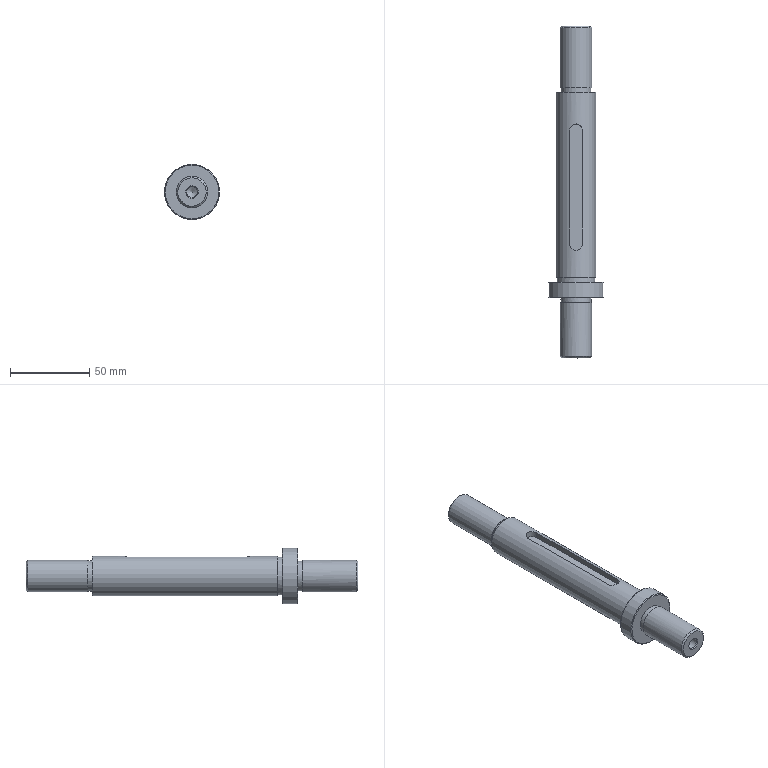Part | STEP file | 冲床-300配套压波_id574_x_t | 1 solid | 30 faces | box 35 x 210 x 35 mm | volume 89544 mm3 | plane 11 | cylinder 11 | cone 8 | commonest cylinder face diameters 6.8 x2 8.04 x2 19 x2 20 x2 24 x1 25 x1
STEP:
#1=CARTESIAN_POINT('',(1267.,-67.,172.35));
#2=VERTEX_POINT('',#1);
#3=CARTESIAN_POINT('',(1250.,-67.,172.35));
#4=DIRECTION('',(0.,-1.,0.));
#5=DIRECTION('',(1.,0.,0.));
#6=AXIS2_PLACEMENT_3D('',#3,#4,#5);
#7=CIRCLE('',#6,17.);
#8=EDGE_CURVE('',#2,#2,#7,.T.);
#9=ORIENTED_EDGE('',*,*,#8,.T.);
#10=EDGE_LOOP('',(#9));
#11=FACE_BOUND('',#10,.T.);
#12=CARTESIAN_POINT('',(1259.5,-67.,172.35));
#13=VERTEX_POINT('',#12);
#14=CARTESIAN_POINT('',(1250.,-67.,172.35));
#15=DIRECTION('',(0.,-1.,0.));
#16=DIRECTION('',(1.,0.,0.));
#17=AXIS2_PLACEMENT_3D('',#14,#15,#16);
#18=CIRCLE('',#17,9.5);
#19=EDGE_CURVE('',#13,#13,#18,.T.);
#20=ORIENTED_EDGE('',*,*,#19,.F.);
#21=EDGE_LOOP('',(#20));
#22=FACE_BOUND('',#21,.T.);
#23=CARTESIAN_POINT('',(1250.,-67.,172.35));
#24=DIRECTION('',(0.,-1.,0.));
#25=DIRECTION('',(1.,0.,0.));
#26=AXIS2_PLACEMENT_3D('',#23,#24,#25);
#27=PLANE('',#26);
#28=ADVANCED_FACE('',(#11,#22),#27,.T.);
#29=CARTESIAN_POINT('',(1233.,-57.,172.35));
#30=VERTEX_POINT('',#29);
#31=CARTESIAN_POINT('',(1250.,-57.,172.35));
#32=DIRECTION('',(0.,1.,0.));
#33=DIRECTION('',(-1.,0.,0.));
#34=AXIS2_PLACEMENT_3D('',#31,#32,#33);
#35=CIRCLE('',#34,17.);
#36=EDGE_CURVE('',#30,#30,#35,.T.);
#37=ORIENTED_EDGE('',*,*,#36,.T.);
#38=EDGE_LOOP('',(#37));
#39=FACE_BOUND('',#38,.T.);
#40=CARTESIAN_POINT('',(1238.,-57.,172.35));
#41=VERTEX_POINT('',#40);
#42=CARTESIAN_POINT('',(1250.,-57.,172.35));
#43=DIRECTION('',(0.,1.,0.));
#44=DIRECTION('',(-1.,0.,0.));
#45=AXIS2_PLACEMENT_3D('',#42,#43,#44);
#46=CIRCLE('',#45,12.);
#47=EDGE_CURVE('',#41,#41,#46,.T.);
#48=ORIENTED_EDGE('',*,*,#47,.F.);
#49=EDGE_LOOP('',(#48));
#50=FACE_BOUND('',#49,.T.);
#51=CARTESIAN_POINT('',(1250.,-57.,172.35));
#52=DIRECTION('',(0.,1.,0.));
#53=DIRECTION('',(-1.,0.,0.));
#54=AXIS2_PLACEMENT_3D('',#51,#52,#53);
#55=PLANE('',#54);
#56=ADVANCED_FACE('',(#39,#50),#55,.T.);
#57=CARTESIAN_POINT('',(1250.,-66.5,189.85));
#58=VERTEX_POINT('',#57);
#59=CARTESIAN_POINT('',(1250.,-66.5,172.35));
#60=DIRECTION('',(0.,1.,0.));
#61=DIRECTION('',(0.,0.,1.));
#62=AXIS2_PLACEMENT_3D('',#59,#60,#61);
#63=CIRCLE('',#62,17.5);
#64=EDGE_CURVE('',#58,#58,#63,.T.);
#65=ORIENTED_EDGE('',*,*,#64,.T.);
#66=EDGE_LOOP('',(#65));
#67=FACE_BOUND('',#66,.T.);
#68=CARTESIAN_POINT('',(1250.,-57.5,154.85));
#69=VERTEX_POINT('',#68);
#70=CARTESIAN_POINT('',(1250.,-57.5,172.35));
#71=DIRECTION('',(0.,-1.,0.));
#72=DIRECTION('',(0.,0.,-1.));
#73=AXIS2_PLACEMENT_3D('',#70,#71,#72);
#74=CIRCLE('',#73,17.5);
#75=EDGE_CURVE('',#69,#69,#74,.T.);
#76=ORIENTED_EDGE('',*,*,#75,.T.);
#77=EDGE_LOOP('',(#76));
#78=FACE_BOUND('',#77,.T.);
#79=CARTESIAN_POINT('',(1250.,-54.,172.35));
#80=DIRECTION('',(0.,-1.,0.));
#81=DIRECTION('',(1.,0.,0.));
#82=AXIS2_PLACEMENT_3D('',#79,#80,#81);
#83=CYLINDRICAL_SURFACE('',#82,17.5);
#84=ADVANCED_FACE('',(#67,#78),#83,.T.);
#85=ORIENTED_EDGE('',*,*,#8,.F.);
#86=EDGE_LOOP('',(#85));
#87=FACE_BOUND('',#86,.T.);
#88=ORIENTED_EDGE('',*,*,#64,.F.);
#89=EDGE_LOOP('',(#88));
#90=FACE_BOUND('',#89,.T.);
#91=CARTESIAN_POINT('',(1250.,-66.5,172.35));
#92=DIRECTION('',(0.,1.,0.));
#93=DIRECTION('',(0.,0.,1.));
#94=AXIS2_PLACEMENT_3D('',#91,#92,#93);
#95=CONICAL_SURFACE('',#94,17.5,45.);
#96=ADVANCED_FACE('',(#87,#90),#95,.T.);
#97=ORIENTED_EDGE('',*,*,#36,.F.);
#98=EDGE_LOOP('',(#97));
#99=FACE_BOUND('',#98,.T.);
#100=ORIENTED_EDGE('',*,*,#75,.F.);
#101=EDGE_LOOP('',(#100));
#102=FACE_BOUND('',#101,.T.);
#103=CARTESIAN_POINT('',(1250.,-57.5,172.35));
#104=DIRECTION('',(0.,-1.,0.));
#105=DIRECTION('',(0.,0.,-1.));
#106=AXIS2_PLACEMENT_3D('',#103,#104,#105);
#107=CONICAL_SURFACE('',#106,17.5,45.);
#108=ADVANCED_FACE('',(#99,#102),#107,.T.);
#109=CARTESIAN_POINT('',(1250.,-54.,160.35));
#110=VERTEX_POINT('',#109);
#111=CARTESIAN_POINT('',(1250.,-54.,172.35));
#112=DIRECTION('',(0.,-1.,0.));
#113=DIRECTION('',(0.,0.,-1.));
#114=AXIS2_PLACEMENT_3D('',#111,#112,#113);
#115=CIRCLE('',#114,12.);
#116=EDGE_CURVE('',#110,#110,#115,.T.);
#117=ORIENTED_EDGE('',*,*,#116,.F.);
#118=EDGE_LOOP('',(#117));
#119=FACE_BOUND('',#118,.T.);
#120=CARTESIAN_POINT('',(1250.,-54.,159.85));
#121=VERTEX_POINT('',#120);
#122=CARTESIAN_POINT('',(1250.,-54.,172.35));
#123=DIRECTION('',(0.,1.,0.));
#124=DIRECTION('',(0.,0.,-1.));
#125=AXIS2_PLACEMENT_3D('',#122,#123,#124);
#126=CIRCLE('',#125,12.5);
#127=EDGE_CURVE('',#121,#121,#126,.T.);
#128=ORIENTED_EDGE('',*,*,#127,.F.);
#129=EDGE_LOOP('',(#128));
#130=FACE_BOUND('',#129,.T.);
#131=CARTESIAN_POINT('',(1250.,-54.,172.35));
#132=DIRECTION('',(0.,-1.,0.));
#133=DIRECTION('',(0.,0.,-1.));
#134=AXIS2_PLACEMENT_3D('',#131,#132,#133);
#135=PLANE('',#134);
#136=ADVANCED_FACE('',(#119,#130),#135,.T.);
#137=ORIENTED_EDGE('',*,*,#47,.T.);
#138=EDGE_LOOP('',(#137));
#139=FACE_BOUND('',#138,.T.);
#140=ORIENTED_EDGE('',*,*,#116,.T.);
#141=EDGE_LOOP('',(#140));
#142=FACE_BOUND('',#141,.T.);
#143=CARTESIAN_POINT('',(1250.,-57.,172.35));
#144=DIRECTION('',(0.,1.,0.));
#145=DIRECTION('',(0.,0.,1.));
#146=AXIS2_PLACEMENT_3D('',#143,#144,#145);
#147=CYLINDRICAL_SURFACE('',#146,12.);
#148=ADVANCED_FACE('',(#139,#142),#147,.T.);
#149=CARTESIAN_POINT('',(1253.4,89.,172.35));
#150=VERTEX_POINT('',#149);
#151=CARTESIAN_POINT('',(1250.,89.,172.35));
#152=DIRECTION('',(0.,1.,0.));
#153=DIRECTION('',(1.,0.,0.));
#154=AXIS2_PLACEMENT_3D('',#151,#152,#153);
#155=CIRCLE('',#154,3.4);
#156=EDGE_CURVE('',#150,#150,#155,.T.);
#157=ORIENTED_EDGE('',*,*,#156,.T.);
#158=EDGE_LOOP('',(#157));
#159=FACE_BOUND('',#158,.T.);
#160=CARTESIAN_POINT('',(1250.,86.957,172.35));
#161=VERTEX_POINT('',#160);
#162=VERTEX_LOOP('',#161);
#163=FACE_BOUND('',#162,.T.);
#164=CARTESIAN_POINT('',(1250.,89.,172.35));
#165=DIRECTION('',(0.,1.,0.));
#166=DIRECTION('',(-1.,0.,0.));
#167=AXIS2_PLACEMENT_3D('',#164,#165,#166);
#168=CONICAL_SURFACE('',#167,3.4,59.);
#169=ADVANCED_FACE('',(#159,#163),#168,.F.);
#170=CARTESIAN_POINT('',(1250.,104.4,175.75));
#171=VERTEX_POINT('',#170);
#172=CARTESIAN_POINT('',(1250.,104.4,172.35));
#173=DIRECTION('',(0.,1.,0.));
#174=DIRECTION('',(0.,0.,1.));
#175=AXIS2_PLACEMENT_3D('',#172,#173,#174);
#176=CIRCLE('',#175,3.4);
#177=EDGE_CURVE('',#171,#171,#176,.T.);
#178=ORIENTED_EDGE('',*,*,#177,.T.);
#179=EDGE_LOOP('',(#178));
#180=FACE_BOUND('',#179,.T.);
#181=ORIENTED_EDGE('',*,*,#156,.F.);
#182=EDGE_LOOP('',(#181));
#183=FACE_BOUND('',#182,.T.);
#184=CARTESIAN_POINT('',(1250.,105.,172.35));
#185=DIRECTION('',(0.,-1.,0.));
#186=DIRECTION('',(1.,0.,0.));
#187=AXIS2_PLACEMENT_3D('',#184,#185,#186);
#188=CYLINDRICAL_SURFACE('',#187,3.4);
#189=ADVANCED_FACE('',(#180,#183),#188,.F.);
#190=ORIENTED_EDGE('',*,*,#177,.F.);
#191=EDGE_LOOP('',(#190));
#192=FACE_BOUND('',#191,.T.);
#193=CARTESIAN_POINT('',(1246.,105.,172.35));
#194=VERTEX_POINT('',#193);
#195=CARTESIAN_POINT('',(1250.,105.,172.35));
#196=DIRECTION('',(0.,-1.,0.));
#197=DIRECTION('',(-1.,0.,0.));
#198=AXIS2_PLACEMENT_3D('',#195,#196,#197);
#199=CIRCLE('',#198,4.);
#200=EDGE_CURVE('',#194,#194,#199,.T.);
#201=ORIENTED_EDGE('',*,*,#200,.F.);
#202=EDGE_LOOP('',(#201));
#203=FACE_BOUND('',#202,.T.);
#204=CARTESIAN_POINT('',(1250.,105.,172.35));
#205=DIRECTION('',(0.,1.,0.));
#206=DIRECTION('',(0.,0.,1.));
#207=AXIS2_PLACEMENT_3D('',#204,#205,#206);
#208=CONICAL_SURFACE('',#207,4.,45.);
#209=ADVANCED_FACE('',(#192,#203),#208,.F.);
#210=ORIENTED_EDGE('',*,*,#200,.T.);
#211=EDGE_LOOP('',(#210));
#212=FACE_BOUND('',#211,.T.);
#213=CARTESIAN_POINT('',(1241.,105.,172.35));
#214=VERTEX_POINT('',#213);
#215=CARTESIAN_POINT('',(1250.,105.,172.35));
#216=DIRECTION('',(0.,1.,0.));
#217=DIRECTION('',(-1.,0.,0.));
#218=AXIS2_PLACEMENT_3D('',#215,#216,#217);
#219=CIRCLE('',#218,9.);
#220=EDGE_CURVE('',#214,#214,#219,.T.);
#221=ORIENTED_EDGE('',*,*,#220,.T.);
#222=EDGE_LOOP('',(#221));
#223=FACE_BOUND('',#222,.T.);
#224=CARTESIAN_POINT('',(1310.,105.,23.05));
#225=DIRECTION('',(0.,1.,0.));
#226=DIRECTION('',(-1.,0.,0.));
#227=AXIS2_PLACEMENT_3D('',#224,#225,#226);
#228=PLANE('',#227);
#229=ADVANCED_FACE('',(#212,#223),#228,.T.);
#230=CARTESIAN_POINT('',(1250.,104.,162.35));
#231=VERTEX_POINT('',#230);
#232=CARTESIAN_POINT('',(1250.,104.,172.35));
#233=DIRECTION('',(0.,-1.,0.));
#234=DIRECTION('',(0.,0.,-1.));
#235=AXIS2_PLACEMENT_3D('',#232,#233,#234);
#236=CIRCLE('',#235,10.);
#237=EDGE_CURVE('',#231,#231,#236,.T.);
#238=ORIENTED_EDGE('',*,*,#237,.F.);
#239=EDGE_LOOP('',(#238));
#240=FACE_BOUND('',#239,.T.);
#241=ORIENTED_EDGE('',*,*,#220,.F.);
#242=EDGE_LOOP('',(#241));
#243=FACE_BOUND('',#242,.T.);
#244=CARTESIAN_POINT('',(1250.,105.,172.35));
#245=DIRECTION('',(0.,-1.,0.));
#246=DIRECTION('',(0.,0.,-1.));
#247=AXIS2_PLACEMENT_3D('',#244,#245,#246);
#248=CONICAL_SURFACE('',#247,9.,45.);
#249=ADVANCED_FACE('',(#240,#243),#248,.T.);
#250=ORIENTED_EDGE('',*,*,#237,.T.);
#251=EDGE_LOOP('',(#250));
#252=FACE_BOUND('',#251,.T.);
#253=CARTESIAN_POINT('',(1250.,66.,182.35));
#254=VERTEX_POINT('',#253);
#255=CARTESIAN_POINT('',(1250.,66.,172.35));
#256=DIRECTION('',(0.,-1.,0.));
#257=DIRECTION('',(0.,0.,1.));
#258=AXIS2_PLACEMENT_3D('',#255,#256,#257);
#259=CIRCLE('',#258,10.);
#260=EDGE_CURVE('',#254,#254,#259,.T.);
#261=ORIENTED_EDGE('',*,*,#260,.F.);
#262=EDGE_LOOP('',(#261));
#263=FACE_BOUND('',#262,.T.);
#264=CARTESIAN_POINT('',(1250.,92.,172.35));
#265=DIRECTION('',(0.,1.,0.));
#266=DIRECTION('',(1.,0.,0.));
#267=AXIS2_PLACEMENT_3D('',#264,#265,#266);
#268=CYLINDRICAL_SURFACE('',#267,10.);
#269=ADVANCED_FACE('',(#252,#263),#268,.T.);
#270=ORIENTED_EDGE('',*,*,#260,.T.);
#271=EDGE_LOOP('',(#270));
#272=FACE_BOUND('',#271,.T.);
#273=CARTESIAN_POINT('',(1250.,66.,181.85));
#274=VERTEX_POINT('',#273);
#275=CARTESIAN_POINT('',(1250.,66.,172.35));
#276=DIRECTION('',(0.,-1.,0.));
#277=DIRECTION('',(0.,0.,1.));
#278=AXIS2_PLACEMENT_3D('',#275,#276,#277);
#279=CIRCLE('',#278,9.5);
#280=EDGE_CURVE('',#274,#274,#279,.T.);
#281=ORIENTED_EDGE('',*,*,#280,.F.);
#282=EDGE_LOOP('',(#281));
#283=FACE_BOUND('',#282,.T.);
#284=CARTESIAN_POINT('',(1250.,66.,172.35));
#285=DIRECTION('',(0.,1.,0.));
#286=DIRECTION('',(0.,0.,1.));
#287=AXIS2_PLACEMENT_3D('',#284,#285,#286);
#288=PLANE('',#287);
#289=ADVANCED_FACE('',(#272,#283),#288,.F.);
#290=CARTESIAN_POINT('',(1250.,63.,162.85));
#291=VERTEX_POINT('',#290);
#292=CARTESIAN_POINT('',(1250.,63.,172.35));
#293=DIRECTION('',(0.,1.,0.));
#294=DIRECTION('',(0.,0.,-1.));
#295=AXIS2_PLACEMENT_3D('',#292,#293,#294);
#296=CIRCLE('',#295,9.5);
#297=EDGE_CURVE('',#291,#291,#296,.T.);
#298=ORIENTED_EDGE('',*,*,#297,.T.);
#299=EDGE_LOOP('',(#298));
#300=FACE_BOUND('',#299,.T.);
#301=ORIENTED_EDGE('',*,*,#280,.T.);
#302=EDGE_LOOP('',(#301));
#303=FACE_BOUND('',#302,.T.);
#304=CARTESIAN_POINT('',(1250.,92.,172.35));
#305=DIRECTION('',(0.,1.,0.));
#306=DIRECTION('',(0.,0.,1.));
#307=AXIS2_PLACEMENT_3D('',#304,#305,#306);
#308=CYLINDRICAL_SURFACE('',#307,9.5);
#309=ADVANCED_FACE('',(#300,#303),#308,.T.);
#310=CARTESIAN_POINT('',(1254.02,38.98,180.65));
#311=VERTEX_POINT('',#310);
#312=CARTESIAN_POINT('',(1245.98,38.98,180.65));
#313=VERTEX_POINT('',#312);
#314=CARTESIAN_POINT('',(1250.,38.98,180.65));
#315=DIRECTION('',(0.,0.,1.));
#316=DIRECTION('',(1.,0.,0.));
#317=AXIS2_PLACEMENT_3D('',#314,#315,#316);
#318=CIRCLE('',#317,4.02);
#319=EDGE_CURVE('',#311,#313,#318,.T.);
#320=ORIENTED_EDGE('',*,*,#319,.T.);
#321=CARTESIAN_POINT('',(1245.98,-32.98,180.65));
#322=VERTEX_POINT('',#321);
#323=CARTESIAN_POINT('',(1245.98,43.,180.65));
#324=DIRECTION('',(0.,1.,0.));
#325=VECTOR('',#324,1.);
#326=LINE('',#323,#325);
#327=EDGE_CURVE('',#322,#313,#326,.T.);
#328=ORIENTED_EDGE('',*,*,#327,.F.);
#329=CARTESIAN_POINT('',(1254.02,-32.98,180.65));
#330=VERTEX_POINT('',#329);
#331=CARTESIAN_POINT('',(1250.,-32.98,180.65));
#332=DIRECTION('',(0.,0.,1.));
#333=DIRECTION('',(1.,0.,0.));
#334=AXIS2_PLACEMENT_3D('',#331,#332,#333);
#335=CIRCLE('',#334,4.02);
#336=EDGE_CURVE('',#322,#330,#335,.T.);
#337=ORIENTED_EDGE('',*,*,#336,.T.);
#338=CARTESIAN_POINT('',(1254.02,43.,180.65));
#339=DIRECTION('',(0.,1.,0.));
#340=VECTOR('',#339,1.);
#341=LINE('',#338,#340);
#342=EDGE_CURVE('',#330,#311,#341,.T.);
#343=ORIENTED_EDGE('',*,*,#342,.T.);
#344=EDGE_LOOP('',(#320,#328,#337,#343));
#345=FACE_OUTER_BOUND('',#344,.T.);
#346=CARTESIAN_POINT('',(1254.02,43.,180.65));
#347=DIRECTION('',(0.,0.,1.));
#348=DIRECTION('',(1.,0.,0.));
#349=AXIS2_PLACEMENT_3D('',#346,#347,#348);
#350=PLANE('',#349);
#351=ADVANCED_FACE('',(#345),#350,.T.);
#352=CARTESIAN_POINT('',(1250.,63.,159.85));
#353=VERTEX_POINT('',#352);
#354=CARTESIAN_POINT('',(1250.,63.,172.35));
#355=DIRECTION('',(0.,1.,0.));
#356=DIRECTION('',(0.,0.,-1.));
#357=AXIS2_PLACEMENT_3D('',#354,#355,#356);
#358=CIRCLE('',#357,12.5);
#359=EDGE_CURVE('',#353,#353,#358,.T.);
#360=ORIENTED_EDGE('',*,*,#359,.T.);
#361=EDGE_LOOP('',(#360));
#362=FACE_BOUND('',#361,.T.);
#363=ORIENTED_EDGE('',*,*,#297,.F.);
#364=EDGE_LOOP('',(#363));
#365=FACE_BOUND('',#364,.T.);
#366=CARTESIAN_POINT('',(1250.,63.,172.35));
#367=DIRECTION('',(0.,-1.,0.));
#368=DIRECTION('',(0.,0.,1.));
#369=AXIS2_PLACEMENT_3D('',#366,#367,#368);
#370=PLANE('',#369);
#371=ADVANCED_FACE('',(#362,#365),#370,.F.);
#372=CARTESIAN_POINT('',(1254.02,-32.98,184.186));
#373=VERTEX_POINT('',#372);
#374=CARTESIAN_POINT('',(1254.02,-32.98,184.85));
#375=DIRECTION('',(0.,0.,1.));
#376=VECTOR('',#375,1.);
#377=LINE('',#374,#376);
#378=EDGE_CURVE('',#330,#373,#377,.T.);
#379=ORIENTED_EDGE('',*,*,#378,.F.);
#380=ORIENTED_EDGE('',*,*,#336,.F.);
#381=CARTESIAN_POINT('',(1245.98,-32.98,184.186));
#382=VERTEX_POINT('',#381);
#383=CARTESIAN_POINT('',(1245.98,-32.98,180.75));
#384=DIRECTION('',(0.,0.,-1.));
#385=VECTOR('',#384,1.);
#386=LINE('',#383,#385);
#387=EDGE_CURVE('',#382,#322,#386,.T.);
#388=ORIENTED_EDGE('',*,*,#387,.F.);
#389=CARTESIAN_POINT('',(1254.02,-32.98,184.186));
#390=CARTESIAN_POINT('',(1254.02,-33.417,184.186));
#391=CARTESIAN_POINT('',(1253.947,-33.86,184.212));
#392=CARTESIAN_POINT('',(1253.807,-34.271,184.256));
#393=CARTESIAN_POINT('',(1253.668,-34.682,184.301));
#394=CARTESIAN_POINT('',(1253.459,-35.073,184.365));
#395=CARTESIAN_POINT('',(1253.198,-35.416,184.434));
#396=CARTESIAN_POINT('',(1252.928,-35.77,184.505));
#397=CARTESIAN_POINT('',(1252.596,-36.082,184.583));
#398=CARTESIAN_POINT('',(1252.224,-36.328,184.65));
#399=CARTESIAN_POINT('',(1251.844,-36.581,184.719));
#400=CARTESIAN_POINT('',(1251.413,-36.772,184.778));
#401=CARTESIAN_POINT('',(1250.966,-36.882,184.813));
#402=CARTESIAN_POINT('',(1250.535,-36.989,184.846));
#403=CARTESIAN_POINT('',(1250.076,-37.024,184.858));
#404=CARTESIAN_POINT('',(1249.632,-36.983,184.845));
#405=CARTESIAN_POINT('',(1249.204,-36.944,184.832));
#406=CARTESIAN_POINT('',(1248.778,-36.833,184.796));
#407=CARTESIAN_POINT('',(1248.387,-36.662,184.745));
#408=CARTESIAN_POINT('',(1247.99,-36.488,184.694));
#409=CARTESIAN_POINT('',(1247.62,-36.248,184.626));
#410=CARTESIAN_POINT('',(1247.301,-35.959,184.555));
#411=CARTESIAN_POINT('',(1246.969,-35.658,184.482));
#412=CARTESIAN_POINT('',(1246.683,-35.296,184.404));
#413=CARTESIAN_POINT('',(1246.468,-34.9,184.341));
#414=CARTESIAN_POINT('',(1246.251,-34.5,184.277));
#415=CARTESIAN_POINT('',(1246.099,-34.053,184.226));
#416=CARTESIAN_POINT('',(1246.028,-33.599,184.202));
#417=CARTESIAN_POINT('',(1245.996,-33.395,184.191));
#418=CARTESIAN_POINT('',(1245.98,-33.187,184.186));
#419=CARTESIAN_POINT('',(1245.98,-32.98,184.186));
#420=B_SPLINE_CURVE_WITH_KNOTS('',3,(#389,#390,#391,#392,#393,#394,#395,#396,#397,#398,#399,#400,#401,#402,#403,#404,#405,#406,#407,#408,#409,#410,#411,#412,#413,#414,#415,#416,#417,#418,#419),.UNSPECIFIED.,.F.,.F.,(4,3,3,3,3,3,3,3,3,3,4),(0.,0.1036,0.207,0.3138,0.4233,0.5292,0.6311,0.7343,0.8422,0.9514,1.),.UNSPECIFIED.);
#421=EDGE_CURVE('',#373,#382,#420,.T.);
#422=ORIENTED_EDGE('',*,*,#421,.F.);
#423=EDGE_LOOP('',(#379,#380,#388,#422));
#424=FACE_OUTER_BOUND('',#423,.T.);
#425=CARTESIAN_POINT('',(1250.,-32.98,184.85));
#426=DIRECTION('',(0.,0.,-1.));
#427=DIRECTION('',(-1.,0.,0.));
#428=AXIS2_PLACEMENT_3D('',#425,#426,#427);
#429=CYLINDRICAL_SURFACE('',#428,4.02);
#430=ADVANCED_FACE('',(#424),#429,.F.);
#431=CARTESIAN_POINT('',(1254.02,38.98,184.186));
#432=VERTEX_POINT('',#431);
#433=CARTESIAN_POINT('',(1254.02,3.,184.186));
#434=DIRECTION('',(0.,1.,0.));
#435=VECTOR('',#434,1.);
#436=LINE('',#433,#435);
#437=EDGE_CURVE('',#373,#432,#436,.T.);
#438=ORIENTED_EDGE('',*,*,#437,.T.);
#439=CARTESIAN_POINT('',(1254.02,38.98,184.85));
#440=DIRECTION('',(0.,0.,-1.));
#441=VECTOR('',#440,1.);
#442=LINE('',#439,#441);
#443=EDGE_CURVE('',#432,#311,#442,.T.);
#444=ORIENTED_EDGE('',*,*,#443,.T.);
#445=ORIENTED_EDGE('',*,*,#342,.F.);
#446=ORIENTED_EDGE('',*,*,#378,.T.);
#447=EDGE_LOOP('',(#438,#444,#445,#446));
#448=FACE_OUTER_BOUND('',#447,.T.);
#449=CARTESIAN_POINT('',(1254.02,43.,184.85));
#450=DIRECTION('',(-1.,0.,0.));
#451=DIRECTION('',(0.,0.,1.));
#452=AXIS2_PLACEMENT_3D('',#449,#450,#451);
#453=PLANE('',#452);
#454=ADVANCED_FACE('',(#448),#453,.T.);
#455=CARTESIAN_POINT('',(1245.98,38.98,184.186));
#456=VERTEX_POINT('',#455);
#457=CARTESIAN_POINT('',(1245.98,38.98,180.75));
#458=DIRECTION('',(0.,0.,1.));
#459=VECTOR('',#458,1.);
#460=LINE('',#457,#459);
#461=EDGE_CURVE('',#313,#456,#460,.T.);
#462=ORIENTED_EDGE('',*,*,#461,.F.);
#463=ORIENTED_EDGE('',*,*,#319,.F.);
#464=ORIENTED_EDGE('',*,*,#443,.F.);
#465=CARTESIAN_POINT('',(1245.98,38.98,184.186));
#466=CARTESIAN_POINT('',(1245.98,39.417,184.186));
#467=CARTESIAN_POINT('',(1246.053,39.86,184.212));
#468=CARTESIAN_POINT('',(1246.193,40.271,184.256));
#469=CARTESIAN_POINT('',(1246.332,40.682,184.301));
#470=CARTESIAN_POINT('',(1246.541,41.073,184.365));
#471=CARTESIAN_POINT('',(1246.802,41.416,184.434));
#472=CARTESIAN_POINT('',(1247.072,41.77,184.505));
#473=CARTESIAN_POINT('',(1247.404,42.082,184.583));
#474=CARTESIAN_POINT('',(1247.776,42.328,184.65));
#475=CARTESIAN_POINT('',(1248.156,42.581,184.719));
#476=CARTESIAN_POINT('',(1248.587,42.772,184.778));
#477=CARTESIAN_POINT('',(1249.034,42.882,184.813));
#478=CARTESIAN_POINT('',(1249.465,42.989,184.846));
#479=CARTESIAN_POINT('',(1249.924,43.024,184.858));
#480=CARTESIAN_POINT('',(1250.368,42.983,184.845));
#481=CARTESIAN_POINT('',(1250.796,42.944,184.832));
#482=CARTESIAN_POINT('',(1251.222,42.833,184.796));
#483=CARTESIAN_POINT('',(1251.613,42.662,184.745));
#484=CARTESIAN_POINT('',(1252.01,42.488,184.694));
#485=CARTESIAN_POINT('',(1252.38,42.248,184.626));
#486=CARTESIAN_POINT('',(1252.699,41.959,184.555));
#487=CARTESIAN_POINT('',(1253.031,41.658,184.482));
#488=CARTESIAN_POINT('',(1253.317,41.296,184.404));
#489=CARTESIAN_POINT('',(1253.532,40.9,184.341));
#490=CARTESIAN_POINT('',(1253.749,40.5,184.277));
#491=CARTESIAN_POINT('',(1253.901,40.053,184.226));
#492=CARTESIAN_POINT('',(1253.972,39.599,184.202));
#493=CARTESIAN_POINT('',(1254.004,39.395,184.191));
#494=CARTESIAN_POINT('',(1254.02,39.187,184.186));
#495=CARTESIAN_POINT('',(1254.02,38.98,184.186));
#496=B_SPLINE_CURVE_WITH_KNOTS('',3,(#465,#466,#467,#468,#469,#470,#471,#472,#473,#474,#475,#476,#477,#478,#479,#480,#481,#482,#483,#484,#485,#486,#487,#488,#489,#490,#491,#492,#493,#494,#495),.UNSPECIFIED.,.F.,.F.,(4,3,3,3,3,3,3,3,3,3,4),(0.,0.1036,0.207,0.3138,0.4233,0.5292,0.6311,0.7343,0.8422,0.9514,1.),.UNSPECIFIED.);
#497=EDGE_CURVE('',#456,#432,#496,.T.);
#498=ORIENTED_EDGE('',*,*,#497,.F.);
#499=EDGE_LOOP('',(#462,#463,#464,#498));
#500=FACE_OUTER_BOUND('',#499,.T.);
#501=CARTESIAN_POINT('',(1250.,38.98,68.35));
#502=DIRECTION('',(0.,0.,-1.));
#503=DIRECTION('',(-1.,0.,0.));
#504=AXIS2_PLACEMENT_3D('',#501,#502,#503);
#505=CYLINDRICAL_SURFACE('',#504,4.02);
#506=ADVANCED_FACE('',(#500),#505,.F.);
#507=CARTESIAN_POINT('',(1245.98,3.,184.186));
#508=DIRECTION('',(0.,-1.,0.));
#509=VECTOR('',#508,1.);
#510=LINE('',#507,#509);
#511=EDGE_CURVE('',#456,#382,#510,.T.);
#512=ORIENTED_EDGE('',*,*,#511,.T.);
#513=ORIENTED_EDGE('',*,*,#387,.T.);
#514=ORIENTED_EDGE('',*,*,#327,.T.);
#515=ORIENTED_EDGE('',*,*,#461,.T.);
#516=EDGE_LOOP('',(#512,#513,#514,#515));
#517=FACE_OUTER_BOUND('',#516,.T.);
#518=CARTESIAN_POINT('',(1245.98,43.,180.75));
#519=DIRECTION('',(1.,0.,0.));
#520=DIRECTION('',(0.,0.,-1.));
#521=AXIS2_PLACEMENT_3D('',#518,#519,#520);
#522=PLANE('',#521);
#523=ADVANCED_FACE('',(#517),#522,.T.);
#524=ORIENTED_EDGE('',*,*,#127,.T.);
#525=EDGE_LOOP('',(#524));
#526=FACE_BOUND('',#525,.T.);
#527=ORIENTED_EDGE('',*,*,#511,.F.);
#528=ORIENTED_EDGE('',*,*,#497,.T.);
#529=ORIENTED_EDGE('',*,*,#437,.F.);
#530=ORIENTED_EDGE('',*,*,#421,.T.);
#531=EDGE_LOOP('',(#527,#528,#529,#530));
#532=FACE_BOUND('',#531,.T.);
#533=ORIENTED_EDGE('',*,*,#359,.F.);
#534=EDGE_LOOP('',(#533));
#535=FACE_BOUND('',#534,.T.);
#536=CARTESIAN_POINT('',(1250.,181.,172.35));
#537=DIRECTION('',(0.,-1.,0.));
#538=DIRECTION('',(0.,0.,-1.));
#539=AXIS2_PLACEMENT_3D('',#536,#537,#538);
#540=CYLINDRICAL_SURFACE('',#539,12.5);
#541=ADVANCED_FACE('',(#526,#532,#535),#540,.T.);
#542=CARTESIAN_POINT('',(1250.,-70.,181.85));
#543=VERTEX_POINT('',#542);
#544=CARTESIAN_POINT('',(1250.,-70.,172.35));
#545=DIRECTION('',(0.,1.,0.));
#546=DIRECTION('',(0.,0.,1.));
#547=AXIS2_PLACEMENT_3D('',#544,#545,#546);
#548=CIRCLE('',#547,9.5);
#549=EDGE_CURVE('',#543,#543,#548,.T.);
#550=ORIENTED_EDGE('',*,*,#549,.F.);
#551=EDGE_LOOP('',(#550));
#552=FACE_BOUND('',#551,.T.);
#553=CARTESIAN_POINT('',(1260.,-70.,172.35));
#554=VERTEX_POINT('',#553);
#555=CARTESIAN_POINT('',(1250.,-70.,172.35));
#556=DIRECTION('',(0.,-1.,0.));
#557=DIRECTION('',(1.,0.,0.));
#558=AXIS2_PLACEMENT_3D('',#555,#556,#557);
#559=CIRCLE('',#558,10.);
#560=EDGE_CURVE('',#554,#554,#559,.T.);
#561=ORIENTED_EDGE('',*,*,#560,.F.);
#562=EDGE_LOOP('',(#561));
#563=FACE_BOUND('',#562,.T.);
#564=CARTESIAN_POINT('',(1250.,-70.,172.35));
#565=DIRECTION('',(0.,1.,0.));
#566=DIRECTION('',(0.,0.,1.));
#567=AXIS2_PLACEMENT_3D('',#564,#565,#566);
#568=PLANE('',#567);
#569=ADVANCED_FACE('',(#552,#563),#568,.T.);
#570=ORIENTED_EDGE('',*,*,#19,.T.);
#571=EDGE_LOOP('',(#570));
#572=FACE_BOUND('',#571,.T.);
#573=ORIENTED_EDGE('',*,*,#549,.T.);
#574=EDGE_LOOP('',(#573));
#575=FACE_BOUND('',#574,.T.);
#576=CARTESIAN_POINT('',(1250.,-67.,172.35));
#577=DIRECTION('',(0.,-1.,0.));
#578=DIRECTION('',(0.,0.,-1.));
#579=AXIS2_PLACEMENT_3D('',#576,#577,#578);
#580=CYLINDRICAL_SURFACE('',#579,9.5);
#581=ADVANCED_FACE('',(#572,#575),#580,.T.);
#582=CARTESIAN_POINT('',(1246.6,-89.,172.35));
#583=VERTEX_POINT('',#582);
#584=CARTESIAN_POINT('',(1250.,-89.,172.35));
#585=DIRECTION('',(0.,-1.,0.));
#586=DIRECTION('',(-1.,0.,0.));
#587=AXIS2_PLACEMENT_3D('',#584,#585,#586);
#588=CIRCLE('',#587,3.4);
#589=EDGE_CURVE('',#583,#583,#588,.T.);
#590=ORIENTED_EDGE('',*,*,#589,.T.);
#591=EDGE_LOOP('',(#590));
#592=FACE_BOUND('',#591,.T.);
#593=CARTESIAN_POINT('',(1250.,-86.957,172.35));
#594=VERTEX_POINT('',#593);
#595=VERTEX_LOOP('',#594);
#596=FACE_BOUND('',#595,.T.);
#597=CARTESIAN_POINT('',(1250.,-89.,172.35));
#598=DIRECTION('',(0.,-1.,0.));
#599=DIRECTION('',(1.,0.,0.));
#600=AXIS2_PLACEMENT_3D('',#597,#598,#599);
#601=CONICAL_SURFACE('',#600,3.4,59.);
#602=ADVANCED_FACE('',(#592,#596),#601,.F.);
#603=CARTESIAN_POINT('',(1250.,-104.4,168.95));
#604=VERTEX_POINT('',#603);
#605=CARTESIAN_POINT('',(1250.,-104.4,172.35));
#606=DIRECTION('',(0.,-1.,0.));
#607=DIRECTION('',(0.,0.,-1.));
#608=AXIS2_PLACEMENT_3D('',#605,#606,#607);
#609=CIRCLE('',#608,3.4);
#610=EDGE_CURVE('',#604,#604,#609,.T.);
#611=ORIENTED_EDGE('',*,*,#610,.T.);
#612=EDGE_LOOP('',(#611));
#613=FACE_BOUND('',#612,.T.);
#614=ORIENTED_EDGE('',*,*,#589,.F.);
#615=EDGE_LOOP('',(#614));
#616=FACE_BOUND('',#615,.T.);
#617=CARTESIAN_POINT('',(1250.,-105.,172.35));
#618=DIRECTION('',(0.,1.,0.));
#619=DIRECTION('',(-1.,0.,0.));
#620=AXIS2_PLACEMENT_3D('',#617,#618,#619);
#621=CYLINDRICAL_SURFACE('',#620,3.4);
#622=ADVANCED_FACE('',(#613,#616),#621,.F.);
#623=ORIENTED_EDGE('',*,*,#610,.F.);
#624=EDGE_LOOP('',(#623));
#625=FACE_BOUND('',#624,.T.);
#626=CARTESIAN_POINT('',(1254.,-105.,172.35));
#627=VERTEX_POINT('',#626);
#628=CARTESIAN_POINT('',(1250.,-105.,172.35));
#629=DIRECTION('',(0.,1.,0.));
#630=DIRECTION('',(1.,0.,0.));
#631=AXIS2_PLACEMENT_3D('',#628,#629,#630);
#632=CIRCLE('',#631,4.);
#633=EDGE_CURVE('',#627,#627,#632,.T.);
#634=ORIENTED_EDGE('',*,*,#633,.F.);
#635=EDGE_LOOP('',(#634));
#636=FACE_BOUND('',#635,.T.);
#637=CARTESIAN_POINT('',(1250.,-105.,172.35));
#638=DIRECTION('',(0.,-1.,0.));
#639=DIRECTION('',(0.,0.,-1.));
#640=AXIS2_PLACEMENT_3D('',#637,#638,#639);
#641=CONICAL_SURFACE('',#640,4.,45.);
#642=ADVANCED_FACE('',(#625,#636),#641,.F.);
#643=ORIENTED_EDGE('',*,*,#633,.T.);
#644=EDGE_LOOP('',(#643));
#645=FACE_BOUND('',#644,.T.);
#646=CARTESIAN_POINT('',(1259.,-105.,172.35));
#647=VERTEX_POINT('',#646);
#648=CARTESIAN_POINT('',(1250.,-105.,172.35));
#649=DIRECTION('',(0.,-1.,0.));
#650=DIRECTION('',(1.,0.,0.));
#651=AXIS2_PLACEMENT_3D('',#648,#649,#650);
#652=CIRCLE('',#651,9.);
#653=EDGE_CURVE('',#647,#647,#652,.T.);
#654=ORIENTED_EDGE('',*,*,#653,.T.);
#655=EDGE_LOOP('',(#654));
#656=FACE_BOUND('',#655,.T.);
#657=CARTESIAN_POINT('',(1310.,-105.,23.05));
#658=DIRECTION('',(0.,-1.,0.));
#659=DIRECTION('',(-1.,0.,0.));
#660=AXIS2_PLACEMENT_3D('',#657,#658,#659);
#661=PLANE('',#660);
#662=ADVANCED_FACE('',(#645,#656),#661,.T.);
#663=CARTESIAN_POINT('',(1250.,-104.,182.35));
#664=VERTEX_POINT('',#663);
#665=CARTESIAN_POINT('',(1250.,-104.,172.35));
#666=DIRECTION('',(0.,1.,0.));
#667=DIRECTION('',(0.,0.,1.));
#668=AXIS2_PLACEMENT_3D('',#665,#666,#667);
#669=CIRCLE('',#668,10.);
#670=EDGE_CURVE('',#664,#664,#669,.T.);
#671=ORIENTED_EDGE('',*,*,#670,.F.);
#672=EDGE_LOOP('',(#671));
#673=FACE_BOUND('',#672,.T.);
#674=ORIENTED_EDGE('',*,*,#653,.F.);
#675=EDGE_LOOP('',(#674));
#676=FACE_BOUND('',#675,.T.);
#677=CARTESIAN_POINT('',(1250.,-105.,172.35));
#678=DIRECTION('',(0.,1.,0.));
#679=DIRECTION('',(0.,0.,1.));
#680=AXIS2_PLACEMENT_3D('',#677,#678,#679);
#681=CONICAL_SURFACE('',#680,9.,45.);
#682=ADVANCED_FACE('',(#673,#676),#681,.T.);
#683=ORIENTED_EDGE('',*,*,#670,.T.);
#684=EDGE_LOOP('',(#683));
#685=FACE_BOUND('',#684,.T.);
#686=ORIENTED_EDGE('',*,*,#560,.T.);
#687=EDGE_LOOP('',(#686));
#688=FACE_BOUND('',#687,.T.);
#689=CARTESIAN_POINT('',(1250.,-70.,172.35));
#690=DIRECTION('',(0.,-1.,0.));
#691=DIRECTION('',(1.,0.,0.));
#692=AXIS2_PLACEMENT_3D('',#689,#690,#691);
#693=CYLINDRICAL_SURFACE('',#692,10.);
#694=ADVANCED_FACE('',(#685,#688),#693,.T.);
#695=CLOSED_SHELL('',(#28,#56,#84,#96,#108,#136,#148,#169,#189,#209,#229,#249,#269,#289,#309,#351,#371,#430,#454,#506,#523,#541,#569,#581,#602,#622,#642,#662,#682,#694));
#696=MANIFOLD_SOLID_BREP('',#695);
#697=(LENGTH_UNIT()NAMED_UNIT(*)SI_UNIT(.MILLI.,.METRE.));
#698=UNCERTAINTY_MEASURE_WITH_UNIT(LENGTH_MEASURE(0.0508),#697,'','');
#699=(NAMED_UNIT(*)PLANE_ANGLE_UNIT()SI_UNIT($,.RADIAN.));
#700=PLANE_ANGLE_MEASURE_WITH_UNIT(PLANE_ANGLE_MEASURE(0.01745),#699);
#701=DIMENSIONAL_EXPONENTS(0.,0.,0.,0.,0.,0.,0.);
#702=(CONVERSION_BASED_UNIT('DEGREE',#700)NAMED_UNIT(#701)PLANE_ANGLE_UNIT());
#703=(NAMED_UNIT(*)SI_UNIT($,.STERADIAN.)SOLID_ANGLE_UNIT());
#704=(GEOMETRIC_REPRESENTATION_CONTEXT(3)GLOBAL_UNCERTAINTY_ASSIGNED_CONTEXT((#698))GLOBAL_UNIT_ASSIGNED_CONTEXT((#697,#702,#703))REPRESENTATION_CONTEXT('',''));
#705=ADVANCED_BREP_SHAPE_REPRESENTATION('',(#696),#704);